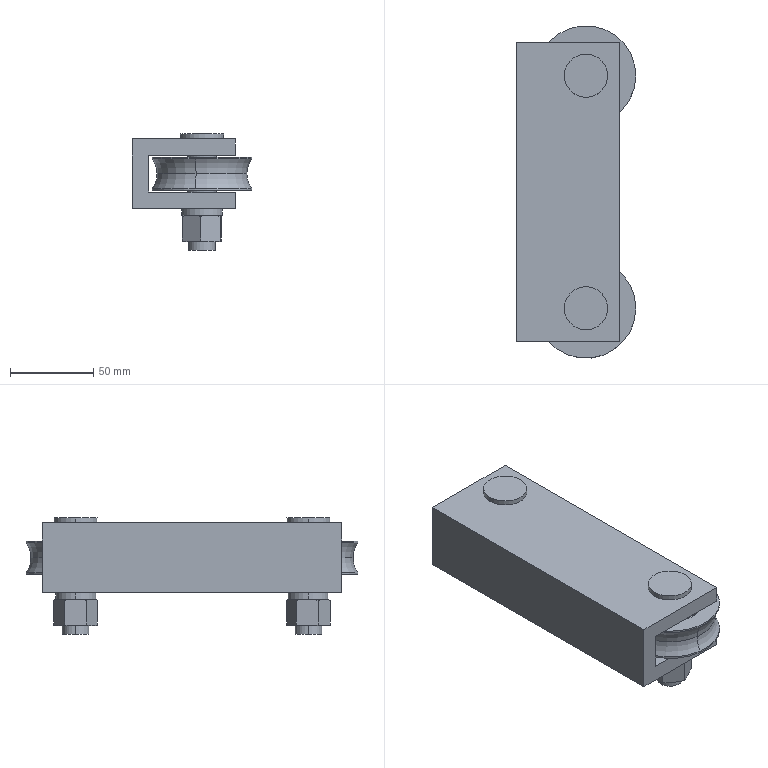Part | SolidWorks | 11 solids | 414 faces | box 72 x 200 x 70 mm | volume 372961 mm3 | cylinder 184 | plane 178 | cone 28 | torus 24 | commonest cylinder face diameters 6.5 x60 22.1 x22 35.1 x22 16 x8 17 x8 17.2 x8